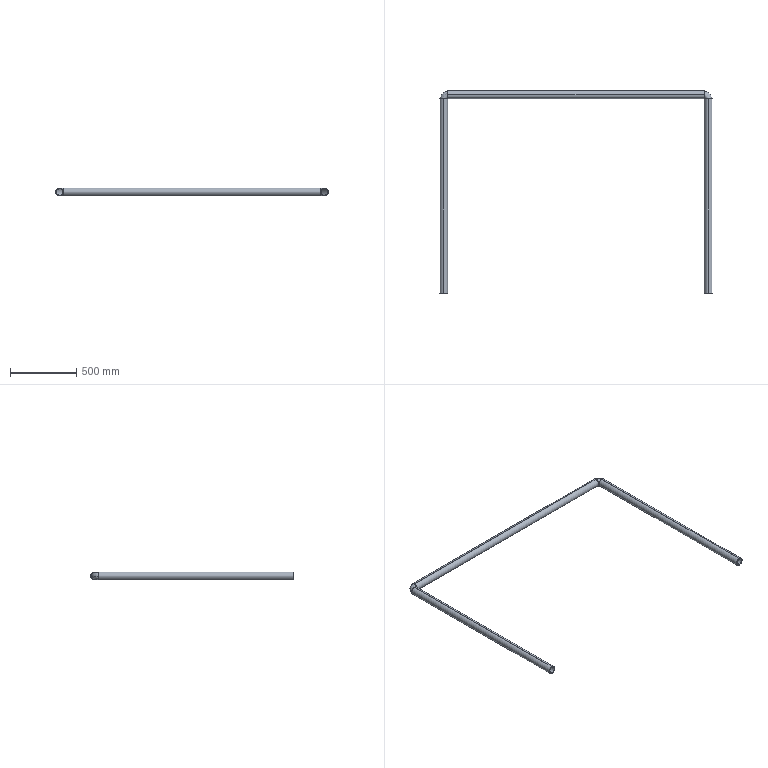Part | SolidWorks | features 3DProfileFeature 1, WeldMemberFeat 1, WeldmentFeature 1 | 5 solids | 28 faces | box 2060 x 1530 x 60 mm | volume 4297442 mm3 | cylinder 12 | plane 10 | torus 6 | commonest cylinder face diameters 50 x6 60 x6
STEP:
#1=CARTESIAN_POINT('',(0.,1470.,30.));
#2=VERTEX_POINT('',#1);
#3=CARTESIAN_POINT('',(0.,1470.,-30.));
#4=VERTEX_POINT('',#3);
#5=CARTESIAN_POINT('',(0.,1470.,0.));
#6=DIRECTION('',(0.,1.,0.));
#7=DIRECTION('',(0.,0.,1.));
#8=AXIS2_PLACEMENT_3D('',#5,#6,#7);
#9=CIRCLE('',#8,30.);
#10=EDGE_CURVE('',#2,#4,#9,.T.);
#11=ORIENTED_EDGE('',*,*,#10,.F.);
#12=CARTESIAN_POINT('',(0.,0.,30.));
#13=VERTEX_POINT('',#12);
#14=CARTESIAN_POINT('',(0.,1470.,30.));
#15=DIRECTION('',(0.,-1.,0.));
#16=VECTOR('',#15,1000.);
#17=LINE('',#14,#16);
#18=EDGE_CURVE('',#2,#13,#17,.T.);
#19=ORIENTED_EDGE('',*,*,#18,.T.);
#20=CARTESIAN_POINT('',(0.,0.,-30.));
#21=VERTEX_POINT('',#20);
#22=CARTESIAN_POINT('',(0.,0.,0.));
#23=DIRECTION('',(0.,1.,0.));
#24=DIRECTION('',(0.,0.,1.));
#25=AXIS2_PLACEMENT_3D('',#22,#23,#24);
#26=CIRCLE('',#25,30.);
#27=EDGE_CURVE('',#13,#21,#26,.T.);
#28=ORIENTED_EDGE('',*,*,#27,.T.);
#29=CARTESIAN_POINT('',(0.,1470.,-30.));
#30=DIRECTION('',(0.,-1.,0.));
#31=VECTOR('',#30,1000.);
#32=LINE('',#29,#31);
#33=EDGE_CURVE('',#4,#21,#32,.T.);
#34=ORIENTED_EDGE('',*,*,#33,.F.);
#35=EDGE_LOOP('',(#11,#19,#28,#34));
#36=FACE_OUTER_BOUND('',#35,.T.);
#37=CARTESIAN_POINT('',(0.,1470.,0.));
#38=DIRECTION('',(0.,-1.,0.));
#39=DIRECTION('',(0.,0.,-1.));
#40=AXIS2_PLACEMENT_3D('',#37,#38,#39);
#41=CYLINDRICAL_SURFACE('',#40,30.);
#42=ADVANCED_FACE('',(#36),#41,.T.);
#43=CARTESIAN_POINT('',(0.,1470.,-25.));
#44=VERTEX_POINT('',#43);
#45=CARTESIAN_POINT('',(0.,1470.,25.));
#46=VERTEX_POINT('',#45);
#47=CARTESIAN_POINT('',(0.,1470.,0.));
#48=DIRECTION('',(0.,1.,0.));
#49=DIRECTION('',(0.,0.,1.));
#50=AXIS2_PLACEMENT_3D('',#47,#48,#49);
#51=CIRCLE('',#50,25.);
#52=EDGE_CURVE('',#44,#46,#51,.T.);
#53=ORIENTED_EDGE('',*,*,#52,.T.);
#54=CARTESIAN_POINT('',(0.,0.,25.));
#55=VERTEX_POINT('',#54);
#56=CARTESIAN_POINT('',(0.,1470.,25.));
#57=DIRECTION('',(0.,-1.,0.));
#58=VECTOR('',#57,1000.);
#59=LINE('',#56,#58);
#60=EDGE_CURVE('',#46,#55,#59,.T.);
#61=ORIENTED_EDGE('',*,*,#60,.T.);
#62=CARTESIAN_POINT('',(0.,0.,-25.));
#63=VERTEX_POINT('',#62);
#64=CARTESIAN_POINT('',(0.,0.,0.));
#65=DIRECTION('',(0.,1.,0.));
#66=DIRECTION('',(0.,0.,1.));
#67=AXIS2_PLACEMENT_3D('',#64,#65,#66);
#68=CIRCLE('',#67,25.);
#69=EDGE_CURVE('',#63,#55,#68,.T.);
#70=ORIENTED_EDGE('',*,*,#69,.F.);
#71=CARTESIAN_POINT('',(0.,1470.,-25.));
#72=DIRECTION('',(0.,-1.,0.));
#73=VECTOR('',#72,1000.);
#74=LINE('',#71,#73);
#75=EDGE_CURVE('',#44,#63,#74,.T.);
#76=ORIENTED_EDGE('',*,*,#75,.F.);
#77=EDGE_LOOP('',(#53,#61,#70,#76));
#78=FACE_OUTER_BOUND('',#77,.T.);
#79=CARTESIAN_POINT('',(0.,1470.,0.));
#80=DIRECTION('',(0.,-1.,0.));
#81=DIRECTION('',(0.,0.,-1.));
#82=AXIS2_PLACEMENT_3D('',#79,#80,#81);
#83=CYLINDRICAL_SURFACE('',#82,25.);
#84=ADVANCED_FACE('',(#78),#83,.F.);
#85=ORIENTED_EDGE('',*,*,#60,.F.);
#86=CARTESIAN_POINT('',(0.,1470.,0.));
#87=DIRECTION('',(0.,1.,0.));
#88=DIRECTION('',(0.,0.,1.));
#89=AXIS2_PLACEMENT_3D('',#86,#87,#88);
#90=CIRCLE('',#89,25.);
#91=EDGE_CURVE('',#46,#44,#90,.T.);
#92=ORIENTED_EDGE('',*,*,#91,.T.);
#93=ORIENTED_EDGE('',*,*,#75,.T.);
#94=CARTESIAN_POINT('',(0.,0.,0.));
#95=DIRECTION('',(0.,1.,0.));
#96=DIRECTION('',(0.,0.,1.));
#97=AXIS2_PLACEMENT_3D('',#94,#95,#96);
#98=CIRCLE('',#97,25.);
#99=EDGE_CURVE('',#55,#63,#98,.T.);
#100=ORIENTED_EDGE('',*,*,#99,.F.);
#101=EDGE_LOOP('',(#85,#92,#93,#100));
#102=FACE_OUTER_BOUND('',#101,.T.);
#103=CARTESIAN_POINT('',(0.,1470.,0.));
#104=DIRECTION('',(0.,-1.,0.));
#105=DIRECTION('',(0.,0.,-1.));
#106=AXIS2_PLACEMENT_3D('',#103,#104,#105);
#107=CYLINDRICAL_SURFACE('',#106,25.);
#108=ADVANCED_FACE('',(#102),#107,.F.);
#109=ORIENTED_EDGE('',*,*,#18,.F.);
#110=CARTESIAN_POINT('',(0.,1470.,0.));
#111=DIRECTION('',(0.,1.,0.));
#112=DIRECTION('',(0.,0.,1.));
#113=AXIS2_PLACEMENT_3D('',#110,#111,#112);
#114=CIRCLE('',#113,30.);
#115=EDGE_CURVE('',#4,#2,#114,.T.);
#116=ORIENTED_EDGE('',*,*,#115,.F.);
#117=ORIENTED_EDGE('',*,*,#33,.T.);
#118=CARTESIAN_POINT('',(0.,0.,0.));
#119=DIRECTION('',(0.,1.,0.));
#120=DIRECTION('',(0.,0.,1.));
#121=AXIS2_PLACEMENT_3D('',#118,#119,#120);
#122=CIRCLE('',#121,30.);
#123=EDGE_CURVE('',#21,#13,#122,.T.);
#124=ORIENTED_EDGE('',*,*,#123,.T.);
#125=EDGE_LOOP('',(#109,#116,#117,#124));
#126=FACE_OUTER_BOUND('',#125,.T.);
#127=CARTESIAN_POINT('',(0.,1470.,0.));
#128=DIRECTION('',(0.,-1.,0.));
#129=DIRECTION('',(0.,0.,-1.));
#130=AXIS2_PLACEMENT_3D('',#127,#128,#129);
#131=CYLINDRICAL_SURFACE('',#130,30.);
#132=ADVANCED_FACE('',(#126),#131,.T.);
#133=ORIENTED_EDGE('',*,*,#69,.T.);
#134=ORIENTED_EDGE('',*,*,#99,.T.);
#135=EDGE_LOOP('',(#133,#134));
#136=FACE_BOUND('',#135,.T.);
#137=ORIENTED_EDGE('',*,*,#123,.F.);
#138=ORIENTED_EDGE('',*,*,#27,.F.);
#139=EDGE_LOOP('',(#137,#138));
#140=FACE_OUTER_BOUND('',#139,.T.);
#141=CARTESIAN_POINT('',(0.,0.,0.));
#142=DIRECTION('',(0.,1.,0.));
#143=DIRECTION('',(0.,0.,1.));
#144=AXIS2_PLACEMENT_3D('',#141,#142,#143);
#145=PLANE('',#144);
#146=ADVANCED_FACE('',(#136,#140),#145,.F.);
#147=ORIENTED_EDGE('',*,*,#52,.F.);
#148=ORIENTED_EDGE('',*,*,#91,.F.);
#149=EDGE_LOOP('',(#147,#148));
#150=FACE_BOUND('',#149,.T.);
#151=ORIENTED_EDGE('',*,*,#115,.T.);
#152=ORIENTED_EDGE('',*,*,#10,.T.);
#153=EDGE_LOOP('',(#151,#152));
#154=FACE_OUTER_BOUND('',#153,.T.);
#155=CARTESIAN_POINT('',(0.,1470.,0.));
#156=DIRECTION('',(0.,1.,0.));
#157=DIRECTION('',(0.,0.,1.));
#158=AXIS2_PLACEMENT_3D('',#155,#156,#157);
#159=PLANE('',#158);
#160=ADVANCED_FACE('',(#150,#154),#159,.T.);
#161=CLOSED_SHELL('',(#42,#84,#108,#132,#146,#160));
#162=MANIFOLD_SOLID_BREP('',#161);
#163=CARTESIAN_POINT('',(25.,1470.,0.));
#164=VERTEX_POINT('',#163);
#165=CARTESIAN_POINT('',(-25.,1470.,0.));
#166=VERTEX_POINT('',#165);
#167=CARTESIAN_POINT('',(0.,1470.,0.));
#168=DIRECTION('',(0.,-1.,0.));
#169=DIRECTION('',(0.,0.,-1.));
#170=AXIS2_PLACEMENT_3D('',#167,#168,#169);
#171=CIRCLE('',#170,25.);
#172=EDGE_CURVE('',#164,#166,#171,.T.);
#173=ORIENTED_EDGE('',*,*,#172,.T.);
#174=CARTESIAN_POINT('',(30.,1525.,0.));
#175=VERTEX_POINT('',#174);
#176=CARTESIAN_POINT('',(30.,1470.,0.));
#177=DIRECTION('',(0.,0.,-1.));
#178=DIRECTION('',(-1.,0.,0.));
#179=AXIS2_PLACEMENT_3D('',#176,#177,#178);
#180=CIRCLE('',#179,55.);
#181=EDGE_CURVE('',#166,#175,#180,.T.);
#182=ORIENTED_EDGE('',*,*,#181,.T.);
#183=CARTESIAN_POINT('',(30.,1475.,0.));
#184=VERTEX_POINT('',#183);
#185=CARTESIAN_POINT('',(30.,1500.,0.));
#186=DIRECTION('',(1.,0.,0.));
#187=DIRECTION('',(0.,1.,0.));
#188=AXIS2_PLACEMENT_3D('',#185,#186,#187);
#189=CIRCLE('',#188,25.);
#190=EDGE_CURVE('',#175,#184,#189,.T.);
#191=ORIENTED_EDGE('',*,*,#190,.T.);
#192=CARTESIAN_POINT('',(30.,1470.,0.));
#193=DIRECTION('',(0.,0.,-1.));
#194=DIRECTION('',(-1.,0.,0.));
#195=AXIS2_PLACEMENT_3D('',#192,#193,#194);
#196=CIRCLE('',#195,5.);
#197=EDGE_CURVE('',#164,#184,#196,.T.);
#198=ORIENTED_EDGE('',*,*,#197,.F.);
#199=EDGE_LOOP('',(#173,#182,#191,#198));
#200=FACE_OUTER_BOUND('',#199,.T.);
#201=CARTESIAN_POINT('',(30.,1470.,0.));
#202=DIRECTION('',(0.,0.,-1.));
#203=DIRECTION('',(-1.,0.,0.));
#204=AXIS2_PLACEMENT_3D('',#201,#202,#203);
#205=TOROIDAL_SURFACE('',#204,30.,25.);
#206=ADVANCED_FACE('',(#200),#205,.F.);
#207=ORIENTED_EDGE('',*,*,#181,.F.);
#208=CARTESIAN_POINT('',(0.,1470.,0.));
#209=DIRECTION('',(0.,-1.,0.));
#210=DIRECTION('',(0.,0.,-1.));
#211=AXIS2_PLACEMENT_3D('',#208,#209,#210);
#212=CIRCLE('',#211,25.);
#213=EDGE_CURVE('',#166,#164,#212,.T.);
#214=ORIENTED_EDGE('',*,*,#213,.T.);
#215=ORIENTED_EDGE('',*,*,#197,.T.);
#216=CARTESIAN_POINT('',(30.,1500.,0.));
#217=DIRECTION('',(1.,0.,0.));
#218=DIRECTION('',(0.,1.,0.));
#219=AXIS2_PLACEMENT_3D('',#216,#217,#218);
#220=CIRCLE('',#219,25.);
#221=EDGE_CURVE('',#184,#175,#220,.T.);
#222=ORIENTED_EDGE('',*,*,#221,.T.);
#223=EDGE_LOOP('',(#207,#214,#215,#222));
#224=FACE_OUTER_BOUND('',#223,.T.);
#225=CARTESIAN_POINT('',(30.,1470.,0.));
#226=DIRECTION('',(0.,0.,-1.));
#227=DIRECTION('',(-1.,0.,0.));
#228=AXIS2_PLACEMENT_3D('',#225,#226,#227);
#229=TOROIDAL_SURFACE('',#228,30.,25.);
#230=ADVANCED_FACE('',(#224),#229,.F.);
#231=ORIENTED_EDGE('',*,*,#221,.F.);
#232=ORIENTED_EDGE('',*,*,#190,.F.);
#233=EDGE_LOOP('',(#231,#232));
#234=FACE_BOUND('',#233,.T.);
#235=CARTESIAN_POINT('',(30.,1470.,0.));
#236=VERTEX_POINT('',#235);
#237=CARTESIAN_POINT('',(30.,1530.,0.));
#238=VERTEX_POINT('',#237);
#239=CARTESIAN_POINT('',(30.,1500.,0.));
#240=DIRECTION('',(-1.,0.,0.));
#241=DIRECTION('',(0.,1.,0.));
#242=AXIS2_PLACEMENT_3D('',#239,#240,#241);
#243=CIRCLE('',#242,30.);
#244=EDGE_CURVE('',#236,#238,#243,.T.);
#245=ORIENTED_EDGE('',*,*,#244,.F.);
#246=CARTESIAN_POINT('',(30.,1500.,0.));
#247=DIRECTION('',(-1.,0.,0.));
#248=DIRECTION('',(0.,1.,0.));
#249=AXIS2_PLACEMENT_3D('',#246,#247,#248);
#250=CIRCLE('',#249,30.);
#251=EDGE_CURVE('',#238,#236,#250,.T.);
#252=ORIENTED_EDGE('',*,*,#251,.F.);
#253=EDGE_LOOP('',(#245,#252));
#254=FACE_OUTER_BOUND('',#253,.T.);
#255=CARTESIAN_POINT('',(30.,1500.,0.));
#256=DIRECTION('',(1.,0.,0.));
#257=DIRECTION('',(0.,1.,0.));
#258=AXIS2_PLACEMENT_3D('',#255,#256,#257);
#259=PLANE('',#258);
#260=ADVANCED_FACE('',(#234,#254),#259,.T.);
#261=ORIENTED_EDGE('',*,*,#244,.T.);
#262=ORIENTED_EDGE('',*,*,#251,.T.);
#263=CARTESIAN_POINT('',(-30.,1470.,0.));
#264=VERTEX_POINT('',#263);
#265=CARTESIAN_POINT('',(0.,1470.,0.));
#266=DIRECTION('',(0.,1.,0.));
#267=DIRECTION('',(0.,0.,-1.));
#268=AXIS2_PLACEMENT_3D('',#265,#266,#267);
#269=CIRCLE('',#268,30.);
#270=EDGE_CURVE('',#236,#264,#269,.T.);
#271=ORIENTED_EDGE('',*,*,#270,.T.);
#272=CARTESIAN_POINT('',(0.,1470.,0.));
#273=DIRECTION('',(0.,1.,0.));
#274=DIRECTION('',(0.,0.,-1.));
#275=AXIS2_PLACEMENT_3D('',#272,#273,#274);
#276=CIRCLE('',#275,30.);
#277=EDGE_CURVE('',#264,#236,#276,.T.);
#278=ORIENTED_EDGE('',*,*,#277,.T.);
#279=EDGE_LOOP('',(#261,#262,#271,#278));
#280=FACE_OUTER_BOUND('',#279,.T.);
#281=CARTESIAN_POINT('',(30.,1470.,0.));
#282=DIRECTION('',(0.,0.,-1.));
#283=DIRECTION('',(-1.,0.,0.));
#284=AXIS2_PLACEMENT_3D('',#281,#282,#283);
#285=TOROIDAL_SURFACE('',#284,30.,30.);
#286=ADVANCED_FACE('',(#280),#285,.T.);
#287=ORIENTED_EDGE('',*,*,#172,.F.);
#288=ORIENTED_EDGE('',*,*,#213,.F.);
#289=EDGE_LOOP('',(#287,#288));
#290=FACE_BOUND('',#289,.T.);
#291=ORIENTED_EDGE('',*,*,#270,.F.);
#292=ORIENTED_EDGE('',*,*,#277,.F.);
#293=EDGE_LOOP('',(#291,#292));
#294=FACE_OUTER_BOUND('',#293,.T.);
#295=CARTESIAN_POINT('',(0.,1470.,0.));
#296=DIRECTION('',(0.,-1.,0.));
#297=DIRECTION('',(0.,0.,-1.));
#298=AXIS2_PLACEMENT_3D('',#295,#296,#297);
#299=PLANE('',#298);
#300=ADVANCED_FACE('',(#290,#294),#299,.T.);
#301=CLOSED_SHELL('',(#206,#230,#260,#286,#300));
#302=MANIFOLD_SOLID_BREP('',#301);
#303=CARTESIAN_POINT('',(1970.,1500.,-30.));
#304=VERTEX_POINT('',#303);
#305=CARTESIAN_POINT('',(1970.,1500.,30.));
#306=VERTEX_POINT('',#305);
#307=CARTESIAN_POINT('',(1970.,1500.,0.));
#308=DIRECTION('',(1.,0.,0.));
#309=DIRECTION('',(0.,1.,0.));
#310=AXIS2_PLACEMENT_3D('',#307,#308,#309);
#311=CIRCLE('',#310,30.);
#312=EDGE_CURVE('',#304,#306,#311,.T.);
#313=ORIENTED_EDGE('',*,*,#312,.F.);
#314=CARTESIAN_POINT('',(30.,1500.,-30.));
#315=VERTEX_POINT('',#314);
#316=CARTESIAN_POINT('',(1970.,1500.,-30.));
#317=DIRECTION('',(-1.,0.,0.));
#318=VECTOR('',#317,1000.);
#319=LINE('',#316,#318);
#320=EDGE_CURVE('',#304,#315,#319,.T.);
#321=ORIENTED_EDGE('',*,*,#320,.T.);
#322=CARTESIAN_POINT('',(30.,1500.,30.));
#323=VERTEX_POINT('',#322);
#324=CARTESIAN_POINT('',(30.,1500.,0.));
#325=DIRECTION('',(-1.,0.,0.));
#326=DIRECTION('',(0.,-1.,0.));
#327=AXIS2_PLACEMENT_3D('',#324,#325,#326);
#328=CIRCLE('',#327,30.);
#329=EDGE_CURVE('',#323,#315,#328,.T.);
#330=ORIENTED_EDGE('',*,*,#329,.F.);
#331=CARTESIAN_POINT('',(1970.,1500.,30.));
#332=DIRECTION('',(-1.,0.,0.));
#333=VECTOR('',#332,1000.);
#334=LINE('',#331,#333);
#335=EDGE_CURVE('',#306,#323,#334,.T.);
#336=ORIENTED_EDGE('',*,*,#335,.F.);
#337=EDGE_LOOP('',(#313,#321,#330,#336));
#338=FACE_OUTER_BOUND('',#337,.T.);
#339=CARTESIAN_POINT('',(1970.,1500.,0.));
#340=DIRECTION('',(-1.,0.,0.));
#341=DIRECTION('',(0.,0.,1.));
#342=AXIS2_PLACEMENT_3D('',#339,#340,#341);
#343=CYLINDRICAL_SURFACE('',#342,30.);
#344=ADVANCED_FACE('',(#338),#343,.T.);
#345=CARTESIAN_POINT('',(1970.,1500.,25.));
#346=VERTEX_POINT('',#345);
#347=CARTESIAN_POINT('',(1970.,1500.,-25.));
#348=VERTEX_POINT('',#347);
#349=CARTESIAN_POINT('',(1970.,1500.,0.));
#350=DIRECTION('',(1.,0.,0.));
#351=DIRECTION('',(0.,1.,0.));
#352=AXIS2_PLACEMENT_3D('',#349,#350,#351);
#353=CIRCLE('',#352,25.);
#354=EDGE_CURVE('',#346,#348,#353,.T.);
#355=ORIENTED_EDGE('',*,*,#354,.T.);
#356=CARTESIAN_POINT('',(30.,1500.,-25.));
#357=VERTEX_POINT('',#356);
#358=CARTESIAN_POINT('',(1970.,1500.,-25.));
#359=DIRECTION('',(-1.,0.,0.));
#360=VECTOR('',#359,1000.);
#361=LINE('',#358,#360);
#362=EDGE_CURVE('',#348,#357,#361,.T.);
#363=ORIENTED_EDGE('',*,*,#362,.T.);
#364=CARTESIAN_POINT('',(30.,1500.,25.));
#365=VERTEX_POINT('',#364);
#366=CARTESIAN_POINT('',(30.,1500.,0.));
#367=DIRECTION('',(-1.,0.,0.));
#368=DIRECTION('',(0.,-1.,0.));
#369=AXIS2_PLACEMENT_3D('',#366,#367,#368);
#370=CIRCLE('',#369,25.);
#371=EDGE_CURVE('',#357,#365,#370,.T.);
#372=ORIENTED_EDGE('',*,*,#371,.T.);
#373=CARTESIAN_POINT('',(1970.,1500.,25.));
#374=DIRECTION('',(-1.,0.,0.));
#375=VECTOR('',#374,1000.);
#376=LINE('',#373,#375);
#377=EDGE_CURVE('',#346,#365,#376,.T.);
#378=ORIENTED_EDGE('',*,*,#377,.F.);
#379=EDGE_LOOP('',(#355,#363,#372,#378));
#380=FACE_OUTER_BOUND('',#379,.T.);
#381=CARTESIAN_POINT('',(1970.,1500.,0.));
#382=DIRECTION('',(-1.,0.,0.));
#383=DIRECTION('',(0.,0.,1.));
#384=AXIS2_PLACEMENT_3D('',#381,#382,#383);
#385=CYLINDRICAL_SURFACE('',#384,25.);
#386=ADVANCED_FACE('',(#380),#385,.F.);
#387=ORIENTED_EDGE('',*,*,#362,.F.);
#388=CARTESIAN_POINT('',(1970.,1500.,0.));
#389=DIRECTION('',(1.,0.,0.));
#390=DIRECTION('',(0.,1.,0.));
#391=AXIS2_PLACEMENT_3D('',#388,#389,#390);
#392=CIRCLE('',#391,25.);
#393=EDGE_CURVE('',#348,#346,#392,.T.);
#394=ORIENTED_EDGE('',*,*,#393,.T.);
#395=ORIENTED_EDGE('',*,*,#377,.T.);
#396=CARTESIAN_POINT('',(30.,1500.,0.));
#397=DIRECTION('',(-1.,0.,0.));
#398=DIRECTION('',(0.,-1.,0.));
#399=AXIS2_PLACEMENT_3D('',#396,#397,#398);
#400=CIRCLE('',#399,25.);
#401=EDGE_CURVE('',#365,#357,#400,.T.);
#402=ORIENTED_EDGE('',*,*,#401,.T.);
#403=EDGE_LOOP('',(#387,#394,#395,#402));
#404=FACE_OUTER_BOUND('',#403,.T.);
#405=CARTESIAN_POINT('',(1970.,1500.,0.));
#406=DIRECTION('',(-1.,0.,0.));
#407=DIRECTION('',(0.,0.,1.));
#408=AXIS2_PLACEMENT_3D('',#405,#406,#407);
#409=CYLINDRICAL_SURFACE('',#408,25.);
#410=ADVANCED_FACE('',(#404),#409,.F.);
#411=ORIENTED_EDGE('',*,*,#320,.F.);
#412=CARTESIAN_POINT('',(1970.,1500.,0.));
#413=DIRECTION('',(1.,0.,0.));
#414=DIRECTION('',(0.,1.,0.));
#415=AXIS2_PLACEMENT_3D('',#412,#413,#414);
#416=CIRCLE('',#415,30.);
#417=EDGE_CURVE('',#306,#304,#416,.T.);
#418=ORIENTED_EDGE('',*,*,#417,.F.);
#419=ORIENTED_EDGE('',*,*,#335,.T.);
#420=CARTESIAN_POINT('',(30.,1500.,0.));
#421=DIRECTION('',(-1.,0.,0.));
#422=DIRECTION('',(0.,-1.,0.));
#423=AXIS2_PLACEMENT_3D('',#420,#421,#422);
#424=CIRCLE('',#423,30.);
#425=EDGE_CURVE('',#315,#323,#424,.T.);
#426=ORIENTED_EDGE('',*,*,#425,.F.);
#427=EDGE_LOOP('',(#411,#418,#419,#426));
#428=FACE_OUTER_BOUND('',#427,.T.);
#429=CARTESIAN_POINT('',(1970.,1500.,0.));
#430=DIRECTION('',(-1.,0.,0.));
#431=DIRECTION('',(0.,0.,1.));
#432=AXIS2_PLACEMENT_3D('',#429,#430,#431);
#433=CYLINDRICAL_SURFACE('',#432,30.);
#434=ADVANCED_FACE('',(#428),#433,.T.);
#435=ORIENTED_EDGE('',*,*,#354,.F.);
#436=ORIENTED_EDGE('',*,*,#393,.F.);
#437=EDGE_LOOP('',(#435,#436));
#438=FACE_BOUND('',#437,.T.);
#439=ORIENTED_EDGE('',*,*,#417,.T.);
#440=ORIENTED_EDGE('',*,*,#312,.T.);
#441=EDGE_LOOP('',(#439,#440));
#442=FACE_OUTER_BOUND('',#441,.T.);
#443=CARTESIAN_POINT('',(1970.,1500.,0.));
#444=DIRECTION('',(1.,0.,0.));
#445=DIRECTION('',(0.,1.,0.));
#446=AXIS2_PLACEMENT_3D('',#443,#444,#445);
#447=PLANE('',#446);
#448=ADVANCED_FACE('',(#438,#442),#447,.T.);
#449=ORIENTED_EDGE('',*,*,#401,.F.);
#450=ORIENTED_EDGE('',*,*,#371,.F.);
#451=EDGE_LOOP('',(#449,#450));
#452=FACE_BOUND('',#451,.T.);
#453=ORIENTED_EDGE('',*,*,#329,.T.);
#454=ORIENTED_EDGE('',*,*,#425,.T.);
#455=EDGE_LOOP('',(#453,#454));
#456=FACE_OUTER_BOUND('',#455,.T.);
#457=CARTESIAN_POINT('',(30.,1500.,0.));
#458=DIRECTION('',(-1.,0.,0.));
#459=DIRECTION('',(0.,-1.,0.));
#460=AXIS2_PLACEMENT_3D('',#457,#458,#459);
#461=PLANE('',#460);
#462=ADVANCED_FACE('',(#452,#456),#461,.T.);
#463=CLOSED_SHELL('',(#344,#386,#410,#434,#448,#462));
#464=MANIFOLD_SOLID_BREP('',#463);
#465=CARTESIAN_POINT('',(2025.,1470.,0.));
#466=VERTEX_POINT('',#465);
#467=CARTESIAN_POINT('',(1975.,1470.,0.));
#468=VERTEX_POINT('',#467);
#469=CARTESIAN_POINT('',(2000.,1470.,0.));
#470=DIRECTION('',(0.,1.,0.));
#471=DIRECTION('',(1.,0.,0.));
#472=AXIS2_PLACEMENT_3D('',#469,#470,#471);
#473=CIRCLE('',#472,25.);
#474=EDGE_CURVE('',#466,#468,#473,.T.);
#475=ORIENTED_EDGE('',*,*,#474,.F.);
#476=CARTESIAN_POINT('',(1970.,1525.,0.));
#477=VERTEX_POINT('',#476);
#478=CARTESIAN_POINT('',(1970.,1470.,0.));
#479=DIRECTION('',(0.,0.,1.));
#480=DIRECTION('',(1.,0.,0.));
#481=AXIS2_PLACEMENT_3D('',#478,#479,#480);
#482=CIRCLE('',#481,55.);
#483=EDGE_CURVE('',#466,#477,#482,.T.);
#484=ORIENTED_EDGE('',*,*,#483,.T.);
#485=CARTESIAN_POINT('',(1970.,1475.,0.));
#486=VERTEX_POINT('',#485);
#487=CARTESIAN_POINT('',(1970.,1500.,0.));
#488=DIRECTION('',(1.,0.,0.));
#489=DIRECTION('',(0.,-1.,0.));
#490=AXIS2_PLACEMENT_3D('',#487,#488,#489);
#491=CIRCLE('',#490,25.);
#492=EDGE_CURVE('',#486,#477,#491,.T.);
#493=ORIENTED_EDGE('',*,*,#492,.F.);
#494=CARTESIAN_POINT('',(1970.,1470.,0.));
#495=DIRECTION('',(0.,0.,1.));
#496=DIRECTION('',(1.,0.,0.));
#497=AXIS2_PLACEMENT_3D('',#494,#495,#496);
#498=CIRCLE('',#497,5.);
#499=EDGE_CURVE('',#468,#486,#498,.T.);
#500=ORIENTED_EDGE('',*,*,#499,.F.);
#501=EDGE_LOOP('',(#475,#484,#493,#500));
#502=FACE_OUTER_BOUND('',#501,.T.);
#503=CARTESIAN_POINT('',(1970.,1470.,0.));
#504=DIRECTION('',(0.,0.,1.));
#505=DIRECTION('',(1.,0.,0.));
#506=AXIS2_PLACEMENT_3D('',#503,#504,#505);
#507=TOROIDAL_SURFACE('',#506,30.,25.);
#508=ADVANCED_FACE('',(#502),#507,.F.);
#509=ORIENTED_EDGE('',*,*,#483,.F.);
#510=CARTESIAN_POINT('',(2000.,1470.,0.));
#511=DIRECTION('',(0.,1.,0.));
#512=DIRECTION('',(1.,0.,0.));
#513=AXIS2_PLACEMENT_3D('',#510,#511,#512);
#514=CIRCLE('',#513,25.);
#515=EDGE_CURVE('',#468,#466,#514,.T.);
#516=ORIENTED_EDGE('',*,*,#515,.F.);
#517=ORIENTED_EDGE('',*,*,#499,.T.);
#518=CARTESIAN_POINT('',(1970.,1500.,0.));
#519=DIRECTION('',(1.,0.,0.));
#520=DIRECTION('',(0.,-1.,0.));
#521=AXIS2_PLACEMENT_3D('',#518,#519,#520);
#522=CIRCLE('',#521,25.);
#523=EDGE_CURVE('',#477,#486,#522,.T.);
#524=ORIENTED_EDGE('',*,*,#523,.F.);
#525=EDGE_LOOP('',(#509,#516,#517,#524));
#526=FACE_OUTER_BOUND('',#525,.T.);
#527=CARTESIAN_POINT('',(1970.,1470.,0.));
#528=DIRECTION('',(0.,0.,1.));
#529=DIRECTION('',(1.,0.,0.));
#530=AXIS2_PLACEMENT_3D('',#527,#528,#529);
#531=TOROIDAL_SURFACE('',#530,30.,25.);
#532=ADVANCED_FACE('',(#526),#531,.F.);
#533=CARTESIAN_POINT('',(1970.,1470.,0.));
#534=VERTEX_POINT('',#533);
#535=CARTESIAN_POINT('',(1970.,1530.,0.));
#536=VERTEX_POINT('',#535);
#537=CARTESIAN_POINT('',(1970.,1500.,0.));
#538=DIRECTION('',(-1.,0.,0.));
#539=DIRECTION('',(0.,-1.,0.));
#540=AXIS2_PLACEMENT_3D('',#537,#538,#539);
#541=CIRCLE('',#540,30.);
#542=EDGE_CURVE('',#534,#536,#541,.T.);
#543=ORIENTED_EDGE('',*,*,#542,.F.);
#544=CARTESIAN_POINT('',(2030.,1470.,0.));
#545=VERTEX_POINT('',#544);
#546=CARTESIAN_POINT('',(2000.,1470.,0.));
#547=DIRECTION('',(0.,-1.,0.));
#548=DIRECTION('',(1.,0.,0.));
#549=AXIS2_PLACEMENT_3D('',#546,#547,#548);
#550=CIRCLE('',#549,30.);
#551=EDGE_CURVE('',#545,#534,#550,.T.);
#552=ORIENTED_EDGE('',*,*,#551,.F.);
#553=CARTESIAN_POINT('',(2000.,1470.,0.));
#554=DIRECTION('',(0.,-1.,0.));
#555=DIRECTION('',(1.,0.,0.));
#556=AXIS2_PLACEMENT_3D('',#553,#554,#555);
#557=CIRCLE('',#556,30.);
#558=EDGE_CURVE('',#534,#545,#557,.T.);
#559=ORIENTED_EDGE('',*,*,#558,.F.);
#560=CARTESIAN_POINT('',(1970.,1500.,0.));
#561=DIRECTION('',(-1.,0.,0.));
#562=DIRECTION('',(0.,-1.,0.));
#563=AXIS2_PLACEMENT_3D('',#560,#561,#562);
#564=CIRCLE('',#563,30.);
#565=EDGE_CURVE('',#536,#534,#564,.T.);
#566=ORIENTED_EDGE('',*,*,#565,.F.);
#567=EDGE_LOOP('',(#543,#552,#559,#566));
#568=FACE_OUTER_BOUND('',#567,.T.);
#569=CARTESIAN_POINT('',(1970.,1470.,0.));
#570=DIRECTION('',(0.,0.,1.));
#571=DIRECTION('',(1.,0.,0.));
#572=AXIS2_PLACEMENT_3D('',#569,#570,#571);
#573=TOROIDAL_SURFACE('',#572,30.,30.);
#574=ADVANCED_FACE('',(#568),#573,.T.);
#575=ORIENTED_EDGE('',*,*,#558,.T.);
#576=ORIENTED_EDGE('',*,*,#551,.T.);
#577=EDGE_LOOP('',(#575,#576));
#578=FACE_OUTER_BOUND('',#577,.T.);
#579=ORIENTED_EDGE('',*,*,#515,.T.);
#580=ORIENTED_EDGE('',*,*,#474,.T.);
#581=EDGE_LOOP('',(#579,#580));
#582=FACE_BOUND('',#581,.T.);
#583=CARTESIAN_POINT('',(2000.,1470.,0.));
#584=DIRECTION('',(0.,-1.,0.));
#585=DIRECTION('',(1.,0.,0.));
#586=AXIS2_PLACEMENT_3D('',#583,#584,#585);
#587=PLANE('',#586);
#588=ADVANCED_FACE('',(#578,#582),#587,.T.);
#589=ORIENTED_EDGE('',*,*,#542,.T.);
#590=ORIENTED_EDGE('',*,*,#565,.T.);
#591=EDGE_LOOP('',(#589,#590));
#592=FACE_OUTER_BOUND('',#591,.T.);
#593=ORIENTED_EDGE('',*,*,#492,.T.);
#594=ORIENTED_EDGE('',*,*,#523,.T.);
#595=EDGE_LOOP('',(#593,#594));
#596=FACE_BOUND('',#595,.T.);
#597=CARTESIAN_POINT('',(1970.,1500.,0.));
#598=DIRECTION('',(-1.,0.,0.));
#599=DIRECTION('',(0.,-1.,0.));
#600=AXIS2_PLACEMENT_3D('',#597,#598,#599);
#601=PLANE('',#600);
#602=ADVANCED_FACE('',(#592,#596),#601,.T.);
#603=CLOSED_SHELL('',(#508,#532,#574,#588,#602));
#604=MANIFOLD_SOLID_BREP('',#603);
#605=CARTESIAN_POINT('',(2000.,0.,-30.));
#606=VERTEX_POINT('',#605);
#607=CARTESIAN_POINT('',(2000.,0.,30.));
#608=VERTEX_POINT('',#607);
#609=CARTESIAN_POINT('',(2000.,0.,0.));
#610=DIRECTION('',(0.,-1.,0.));
#611=DIRECTION('',(0.,0.,1.));
#612=AXIS2_PLACEMENT_3D('',#609,#610,#611);
#613=CIRCLE('',#612,30.);
#614=EDGE_CURVE('',#606,#608,#613,.T.);
#615=ORIENTED_EDGE('',*,*,#614,.F.);
#616=CARTESIAN_POINT('',(2000.,1470.,-30.));
#617=VERTEX_POINT('',#616);
#618=CARTESIAN_POINT('',(2000.,0.,-30.));
#619=DIRECTION('',(0.,1.,0.));
#620=VECTOR('',#619,1000.);
#621=LINE('',#618,#620);
#622=EDGE_CURVE('',#606,#617,#621,.T.);
#623=ORIENTED_EDGE('',*,*,#622,.T.);
#624=CARTESIAN_POINT('',(2000.,1470.,30.));
#625=VERTEX_POINT('',#624);
#626=CARTESIAN_POINT('',(2000.,1470.,0.));
#627=DIRECTION('',(0.,1.,0.));
#628=DIRECTION('',(-1.,0.,0.));
#629=AXIS2_PLACEMENT_3D('',#626,#627,#628);
#630=CIRCLE('',#629,30.);
#631=EDGE_CURVE('',#625,#617,#630,.T.);
#632=ORIENTED_EDGE('',*,*,#631,.F.);
#633=CARTESIAN_POINT('',(2000.,0.,30.));
#634=DIRECTION('',(0.,1.,0.));
#635=VECTOR('',#634,1000.);
#636=LINE('',#633,#635);
#637=EDGE_CURVE('',#608,#625,#636,.T.);
#638=ORIENTED_EDGE('',*,*,#637,.F.);
#639=EDGE_LOOP('',(#615,#623,#632,#638));
#640=FACE_OUTER_BOUND('',#639,.T.);
#641=CARTESIAN_POINT('',(2000.,0.,0.));
#642=DIRECTION('',(0.,1.,0.));
#643=DIRECTION('',(0.,0.,1.));
#644=AXIS2_PLACEMENT_3D('',#641,#642,#643);
#645=CYLINDRICAL_SURFACE('',#644,30.);
#646=ADVANCED_FACE('',(#640),#645,.T.);
#647=CARTESIAN_POINT('',(2000.,0.,25.));
#648=VERTEX_POINT('',#647);
#649=CARTESIAN_POINT('',(2000.,0.,-25.));
#650=VERTEX_POINT('',#649);
#651=CARTESIAN_POINT('',(2000.,0.,0.));
#652=DIRECTION('',(0.,-1.,0.));
#653=DIRECTION('',(0.,0.,1.));
#654=AXIS2_PLACEMENT_3D('',#651,#652,#653);
#655=CIRCLE('',#654,25.);
#656=EDGE_CURVE('',#648,#650,#655,.T.);
#657=ORIENTED_EDGE('',*,*,#656,.T.);
#658=CARTESIAN_POINT('',(2000.,1470.,-25.));
#659=VERTEX_POINT('',#658);
#660=CARTESIAN_POINT('',(2000.,0.,-25.));
#661=DIRECTION('',(0.,1.,0.));
#662=VECTOR('',#661,1000.);
#663=LINE('',#660,#662);
#664=EDGE_CURVE('',#650,#659,#663,.T.);
#665=ORIENTED_EDGE('',*,*,#664,.T.);
#666=CARTESIAN_POINT('',(2000.,1470.,25.));
#667=VERTEX_POINT('',#666);
#668=CARTESIAN_POINT('',(2000.,1470.,0.));
#669=DIRECTION('',(0.,1.,0.));
#670=DIRECTION('',(-1.,0.,0.));
#671=AXIS2_PLACEMENT_3D('',#668,#669,#670);
#672=CIRCLE('',#671,25.);
#673=EDGE_CURVE('',#659,#667,#672,.T.);
#674=ORIENTED_EDGE('',*,*,#673,.T.);
#675=CARTESIAN_POINT('',(2000.,0.,25.));
#676=DIRECTION('',(0.,1.,0.));
#677=VECTOR('',#676,1000.);
#678=LINE('',#675,#677);
#679=EDGE_CURVE('',#648,#667,#678,.T.);
#680=ORIENTED_EDGE('',*,*,#679,.F.);
#681=EDGE_LOOP('',(#657,#665,#674,#680));
#682=FACE_OUTER_BOUND('',#681,.T.);
#683=CARTESIAN_POINT('',(2000.,0.,0.));
#684=DIRECTION('',(0.,1.,0.));
#685=DIRECTION('',(0.,0.,1.));
#686=AXIS2_PLACEMENT_3D('',#683,#684,#685);
#687=CYLINDRICAL_SURFACE('',#686,25.);
#688=ADVANCED_FACE('',(#682),#687,.F.);
#689=ORIENTED_EDGE('',*,*,#664,.F.);
#690=CARTESIAN_POINT('',(2000.,0.,0.));
#691=DIRECTION('',(0.,-1.,0.));
#692=DIRECTION('',(0.,0.,1.));
#693=AXIS2_PLACEMENT_3D('',#690,#691,#692);
#694=CIRCLE('',#693,25.);
#695=EDGE_CURVE('',#650,#648,#694,.T.);
#696=ORIENTED_EDGE('',*,*,#695,.T.);
#697=ORIENTED_EDGE('',*,*,#679,.T.);
#698=CARTESIAN_POINT('',(2000.,1470.,0.));
#699=DIRECTION('',(0.,1.,0.));
#700=DIRECTION('',(-1.,0.,0.));
#701=AXIS2_PLACEMENT_3D('',#698,#699,#700);
#702=CIRCLE('',#701,25.);
#703=EDGE_CURVE('',#667,#659,#702,.T.);
#704=ORIENTED_EDGE('',*,*,#703,.T.);
#705=EDGE_LOOP('',(#689,#696,#697,#704));
#706=FACE_OUTER_BOUND('',#705,.T.);
#707=CARTESIAN_POINT('',(2000.,0.,0.));
#708=DIRECTION('',(0.,1.,0.));
#709=DIRECTION('',(0.,0.,1.));
#710=AXIS2_PLACEMENT_3D('',#707,#708,#709);
#711=CYLINDRICAL_SURFACE('',#710,25.);
#712=ADVANCED_FACE('',(#706),#711,.F.);
#713=ORIENTED_EDGE('',*,*,#622,.F.);
#714=CARTESIAN_POINT('',(2000.,0.,0.));
#715=DIRECTION('',(0.,-1.,0.));
#716=DIRECTION('',(0.,0.,1.));
#717=AXIS2_PLACEMENT_3D('',#714,#715,#716);
#718=CIRCLE('',#717,30.);
#719=EDGE_CURVE('',#608,#606,#718,.T.);
#720=ORIENTED_EDGE('',*,*,#719,.F.);
#721=ORIENTED_EDGE('',*,*,#637,.T.);
#722=CARTESIAN_POINT('',(2000.,1470.,0.));
#723=DIRECTION('',(0.,1.,0.));
#724=DIRECTION('',(-1.,0.,0.));
#725=AXIS2_PLACEMENT_3D('',#722,#723,#724);
#726=CIRCLE('',#725,30.);
#727=EDGE_CURVE('',#617,#625,#726,.T.);
#728=ORIENTED_EDGE('',*,*,#727,.F.);
#729=EDGE_LOOP('',(#713,#720,#721,#728));
#730=FACE_OUTER_BOUND('',#729,.T.);
#731=CARTESIAN_POINT('',(2000.,0.,0.));
#732=DIRECTION('',(0.,1.,0.));
#733=DIRECTION('',(0.,0.,1.));
#734=AXIS2_PLACEMENT_3D('',#731,#732,#733);
#735=CYLINDRICAL_SURFACE('',#734,30.);
#736=ADVANCED_FACE('',(#730),#735,.T.);
#737=ORIENTED_EDGE('',*,*,#656,.F.);
#738=ORIENTED_EDGE('',*,*,#695,.F.);
#739=EDGE_LOOP('',(#737,#738));
#740=FACE_BOUND('',#739,.T.);
#741=ORIENTED_EDGE('',*,*,#719,.T.);
#742=ORIENTED_EDGE('',*,*,#614,.T.);
#743=EDGE_LOOP('',(#741,#742));
#744=FACE_OUTER_BOUND('',#743,.T.);
#745=CARTESIAN_POINT('',(2000.,0.,0.));
#746=DIRECTION('',(0.,-1.,0.));
#747=DIRECTION('',(0.,0.,1.));
#748=AXIS2_PLACEMENT_3D('',#745,#746,#747);
#749=PLANE('',#748);
#750=ADVANCED_FACE('',(#740,#744),#749,.T.);
#751=ORIENTED_EDGE('',*,*,#703,.F.);
#752=ORIENTED_EDGE('',*,*,#673,.F.);
#753=EDGE_LOOP('',(#751,#752));
#754=FACE_BOUND('',#753,.T.);
#755=ORIENTED_EDGE('',*,*,#631,.T.);
#756=ORIENTED_EDGE('',*,*,#727,.T.);
#757=EDGE_LOOP('',(#755,#756));
#758=FACE_OUTER_BOUND('',#757,.T.);
#759=CARTESIAN_POINT('',(2000.,1470.,0.));
#760=DIRECTION('',(0.,1.,0.));
#761=DIRECTION('',(-1.,0.,0.));
#762=AXIS2_PLACEMENT_3D('',#759,#760,#761);
#763=PLANE('',#762);
#764=ADVANCED_FACE('',(#754,#758),#763,.T.);
#765=CLOSED_SHELL('',(#646,#688,#712,#736,#750,#764));
#766=MANIFOLD_SOLID_BREP('',#765);
#767=CARTESIAN_POINT('',(0.,0.,0.));
#768=DIRECTION('',(0.,0.,1.));
#769=DIRECTION('',(1.,0.,0.));
#770=AXIS2_PLACEMENT_3D('',#767,#768,#769);
#771=(LENGTH_UNIT()NAMED_UNIT(*)SI_UNIT(.MILLI.,.METRE.));
#772=UNCERTAINTY_MEASURE_WITH_UNIT(LENGTH_MEASURE(0.00001),#771,'','');
#773=(NAMED_UNIT(*)PLANE_ANGLE_UNIT()SI_UNIT($,.RADIAN.));
#774=(NAMED_UNIT(*)SI_UNIT($,.STERADIAN.)SOLID_ANGLE_UNIT());
#775=(GEOMETRIC_REPRESENTATION_CONTEXT(3)GLOBAL_UNCERTAINTY_ASSIGNED_CONTEXT((#772))GLOBAL_UNIT_ASSIGNED_CONTEXT((#771,#773,#774))REPRESENTATION_CONTEXT('',''));
#776=ADVANCED_BREP_SHAPE_REPRESENTATION('',(#162,#302,#464,#604,#766,#770),#775);